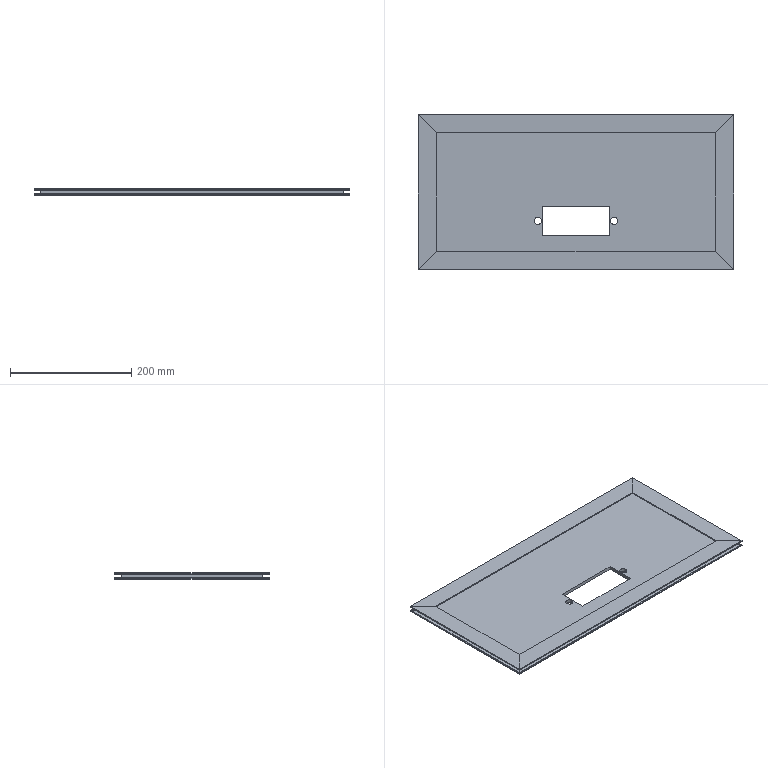Part | SolidWorks | features ICE 2, WeldMemberFeat 1, WeldmentFeature 1 | 5 solids | 102 faces | box 520 x 255 x 10 mm | volume 693362 mm3 | plane 82 | cylinder 20 | commonest cylinder face diameters 2 x16 12 x4